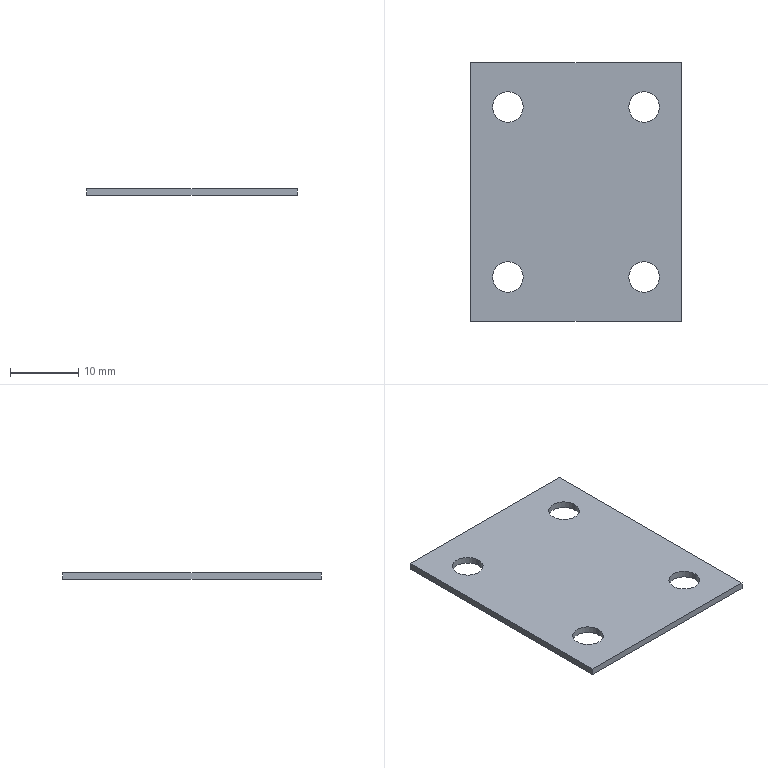Part | SolidWorks | features Extrusion 1 | 1 solid | 14 faces | box 31 x 38 x 1 mm | volume 1114 mm3 | cylinder 8 | plane 6 | commonest cylinder face diameters 4.5 x8
STEP:
#1=CARTESIAN_POINT('',(-12.25,-12.5,1.));
#2=VERTEX_POINT('',#1);
#3=CARTESIAN_POINT('',(-7.75,-12.5,1.));
#4=VERTEX_POINT('',#3);
#5=CARTESIAN_POINT('',(-10.,-12.5,1.));
#6=DIRECTION('',(0.,0.,1.));
#7=DIRECTION('',(1.,0.,0.));
#8=AXIS2_PLACEMENT_3D('',#5,#6,#7);
#9=CIRCLE('',#8,2.25);
#10=EDGE_CURVE('',#2,#4,#9,.T.);
#11=ORIENTED_EDGE('',*,*,#10,.T.);
#12=CARTESIAN_POINT('',(-7.75,-12.5,0.));
#13=VERTEX_POINT('',#12);
#14=CARTESIAN_POINT('',(-7.75,-12.5,1.));
#15=DIRECTION('',(0.,0.,-1.));
#16=VECTOR('',#15,1000.);
#17=LINE('',#14,#16);
#18=EDGE_CURVE('',#4,#13,#17,.T.);
#19=ORIENTED_EDGE('',*,*,#18,.T.);
#20=CARTESIAN_POINT('',(-12.25,-12.5,0.));
#21=VERTEX_POINT('',#20);
#22=CARTESIAN_POINT('',(-10.,-12.5,0.));
#23=DIRECTION('',(0.,0.,1.));
#24=DIRECTION('',(1.,0.,0.));
#25=AXIS2_PLACEMENT_3D('',#22,#23,#24);
#26=CIRCLE('',#25,2.25);
#27=EDGE_CURVE('',#21,#13,#26,.T.);
#28=ORIENTED_EDGE('',*,*,#27,.F.);
#29=CARTESIAN_POINT('',(-12.25,-12.5,1.));
#30=DIRECTION('',(0.,0.,-1.));
#31=VECTOR('',#30,1000.);
#32=LINE('',#29,#31);
#33=EDGE_CURVE('',#2,#21,#32,.T.);
#34=ORIENTED_EDGE('',*,*,#33,.F.);
#35=EDGE_LOOP('',(#11,#19,#28,#34));
#36=FACE_OUTER_BOUND('',#35,.T.);
#37=CARTESIAN_POINT('',(-10.,-12.5,1.));
#38=DIRECTION('',(0.,0.,-1.));
#39=DIRECTION('',(-1.,0.,0.));
#40=AXIS2_PLACEMENT_3D('',#37,#38,#39);
#41=CYLINDRICAL_SURFACE('',#40,2.25);
#42=ADVANCED_FACE('',(#36),#41,.F.);
#43=CARTESIAN_POINT('',(7.75,-12.5,1.));
#44=VERTEX_POINT('',#43);
#45=CARTESIAN_POINT('',(12.25,-12.5,1.));
#46=VERTEX_POINT('',#45);
#47=CARTESIAN_POINT('',(10.,-12.5,1.));
#48=DIRECTION('',(0.,0.,1.));
#49=DIRECTION('',(1.,0.,0.));
#50=AXIS2_PLACEMENT_3D('',#47,#48,#49);
#51=CIRCLE('',#50,2.25);
#52=EDGE_CURVE('',#44,#46,#51,.T.);
#53=ORIENTED_EDGE('',*,*,#52,.T.);
#54=CARTESIAN_POINT('',(12.25,-12.5,0.));
#55=VERTEX_POINT('',#54);
#56=CARTESIAN_POINT('',(12.25,-12.5,1.));
#57=DIRECTION('',(0.,0.,-1.));
#58=VECTOR('',#57,1000.);
#59=LINE('',#56,#58);
#60=EDGE_CURVE('',#46,#55,#59,.T.);
#61=ORIENTED_EDGE('',*,*,#60,.T.);
#62=CARTESIAN_POINT('',(7.75,-12.5,0.));
#63=VERTEX_POINT('',#62);
#64=CARTESIAN_POINT('',(10.,-12.5,0.));
#65=DIRECTION('',(0.,0.,1.));
#66=DIRECTION('',(1.,0.,0.));
#67=AXIS2_PLACEMENT_3D('',#64,#65,#66);
#68=CIRCLE('',#67,2.25);
#69=EDGE_CURVE('',#63,#55,#68,.T.);
#70=ORIENTED_EDGE('',*,*,#69,.F.);
#71=CARTESIAN_POINT('',(7.75,-12.5,1.));
#72=DIRECTION('',(0.,0.,-1.));
#73=VECTOR('',#72,1000.);
#74=LINE('',#71,#73);
#75=EDGE_CURVE('',#44,#63,#74,.T.);
#76=ORIENTED_EDGE('',*,*,#75,.F.);
#77=EDGE_LOOP('',(#53,#61,#70,#76));
#78=FACE_OUTER_BOUND('',#77,.T.);
#79=CARTESIAN_POINT('',(10.,-12.5,1.));
#80=DIRECTION('',(0.,0.,-1.));
#81=DIRECTION('',(-1.,0.,0.));
#82=AXIS2_PLACEMENT_3D('',#79,#80,#81);
#83=CYLINDRICAL_SURFACE('',#82,2.25);
#84=ADVANCED_FACE('',(#78),#83,.F.);
#85=CARTESIAN_POINT('',(7.75,12.5,1.));
#86=VERTEX_POINT('',#85);
#87=CARTESIAN_POINT('',(12.25,12.5,1.));
#88=VERTEX_POINT('',#87);
#89=CARTESIAN_POINT('',(10.,12.5,1.));
#90=DIRECTION('',(0.,0.,1.));
#91=DIRECTION('',(1.,0.,0.));
#92=AXIS2_PLACEMENT_3D('',#89,#90,#91);
#93=CIRCLE('',#92,2.25);
#94=EDGE_CURVE('',#86,#88,#93,.T.);
#95=ORIENTED_EDGE('',*,*,#94,.T.);
#96=CARTESIAN_POINT('',(12.25,12.5,0.));
#97=VERTEX_POINT('',#96);
#98=CARTESIAN_POINT('',(12.25,12.5,1.));
#99=DIRECTION('',(0.,0.,-1.));
#100=VECTOR('',#99,1000.);
#101=LINE('',#98,#100);
#102=EDGE_CURVE('',#88,#97,#101,.T.);
#103=ORIENTED_EDGE('',*,*,#102,.T.);
#104=CARTESIAN_POINT('',(7.75,12.5,0.));
#105=VERTEX_POINT('',#104);
#106=CARTESIAN_POINT('',(10.,12.5,0.));
#107=DIRECTION('',(0.,0.,1.));
#108=DIRECTION('',(1.,0.,0.));
#109=AXIS2_PLACEMENT_3D('',#106,#107,#108);
#110=CIRCLE('',#109,2.25);
#111=EDGE_CURVE('',#105,#97,#110,.T.);
#112=ORIENTED_EDGE('',*,*,#111,.F.);
#113=CARTESIAN_POINT('',(7.75,12.5,1.));
#114=DIRECTION('',(0.,0.,-1.));
#115=VECTOR('',#114,1000.);
#116=LINE('',#113,#115);
#117=EDGE_CURVE('',#86,#105,#116,.T.);
#118=ORIENTED_EDGE('',*,*,#117,.F.);
#119=EDGE_LOOP('',(#95,#103,#112,#118));
#120=FACE_OUTER_BOUND('',#119,.T.);
#121=CARTESIAN_POINT('',(10.,12.5,1.));
#122=DIRECTION('',(0.,0.,-1.));
#123=DIRECTION('',(-1.,0.,0.));
#124=AXIS2_PLACEMENT_3D('',#121,#122,#123);
#125=CYLINDRICAL_SURFACE('',#124,2.25);
#126=ADVANCED_FACE('',(#120),#125,.F.);
#127=CARTESIAN_POINT('',(-12.25,12.5,1.));
#128=VERTEX_POINT('',#127);
#129=CARTESIAN_POINT('',(-7.75,12.5,1.));
#130=VERTEX_POINT('',#129);
#131=CARTESIAN_POINT('',(-10.,12.5,1.));
#132=DIRECTION('',(0.,0.,1.));
#133=DIRECTION('',(1.,0.,0.));
#134=AXIS2_PLACEMENT_3D('',#131,#132,#133);
#135=CIRCLE('',#134,2.25);
#136=EDGE_CURVE('',#128,#130,#135,.T.);
#137=ORIENTED_EDGE('',*,*,#136,.T.);
#138=CARTESIAN_POINT('',(-7.75,12.5,0.));
#139=VERTEX_POINT('',#138);
#140=CARTESIAN_POINT('',(-7.75,12.5,1.));
#141=DIRECTION('',(0.,0.,-1.));
#142=VECTOR('',#141,1000.);
#143=LINE('',#140,#142);
#144=EDGE_CURVE('',#130,#139,#143,.T.);
#145=ORIENTED_EDGE('',*,*,#144,.T.);
#146=CARTESIAN_POINT('',(-12.25,12.5,0.));
#147=VERTEX_POINT('',#146);
#148=CARTESIAN_POINT('',(-10.,12.5,0.));
#149=DIRECTION('',(0.,0.,1.));
#150=DIRECTION('',(1.,0.,0.));
#151=AXIS2_PLACEMENT_3D('',#148,#149,#150);
#152=CIRCLE('',#151,2.25);
#153=EDGE_CURVE('',#147,#139,#152,.T.);
#154=ORIENTED_EDGE('',*,*,#153,.F.);
#155=CARTESIAN_POINT('',(-12.25,12.5,1.));
#156=DIRECTION('',(0.,0.,-1.));
#157=VECTOR('',#156,1000.);
#158=LINE('',#155,#157);
#159=EDGE_CURVE('',#128,#147,#158,.T.);
#160=ORIENTED_EDGE('',*,*,#159,.F.);
#161=EDGE_LOOP('',(#137,#145,#154,#160));
#162=FACE_OUTER_BOUND('',#161,.T.);
#163=CARTESIAN_POINT('',(-10.,12.5,1.));
#164=DIRECTION('',(0.,0.,-1.));
#165=DIRECTION('',(-1.,0.,0.));
#166=AXIS2_PLACEMENT_3D('',#163,#164,#165);
#167=CYLINDRICAL_SURFACE('',#166,2.25);
#168=ADVANCED_FACE('',(#162),#167,.F.);
#169=ORIENTED_EDGE('',*,*,#52,.F.);
#170=CARTESIAN_POINT('',(10.,-12.5,1.));
#171=DIRECTION('',(0.,0.,1.));
#172=DIRECTION('',(1.,0.,0.));
#173=AXIS2_PLACEMENT_3D('',#170,#171,#172);
#174=CIRCLE('',#173,2.25);
#175=EDGE_CURVE('',#46,#44,#174,.T.);
#176=ORIENTED_EDGE('',*,*,#175,.F.);
#177=EDGE_LOOP('',(#169,#176));
#178=FACE_BOUND('',#177,.T.);
#179=ORIENTED_EDGE('',*,*,#136,.F.);
#180=CARTESIAN_POINT('',(-10.,12.5,1.));
#181=DIRECTION('',(0.,0.,1.));
#182=DIRECTION('',(1.,0.,0.));
#183=AXIS2_PLACEMENT_3D('',#180,#181,#182);
#184=CIRCLE('',#183,2.25);
#185=EDGE_CURVE('',#130,#128,#184,.T.);
#186=ORIENTED_EDGE('',*,*,#185,.F.);
#187=EDGE_LOOP('',(#179,#186));
#188=FACE_BOUND('',#187,.T.);
#189=CARTESIAN_POINT('',(-15.5,19.,1.));
#190=VERTEX_POINT('',#189);
#191=CARTESIAN_POINT('',(-15.5,-19.,1.));
#192=VERTEX_POINT('',#191);
#193=CARTESIAN_POINT('',(-15.5,-19.,1.));
#194=DIRECTION('',(0.,-1.,0.));
#195=VECTOR('',#194,1000.);
#196=LINE('',#193,#195);
#197=EDGE_CURVE('',#190,#192,#196,.T.);
#198=ORIENTED_EDGE('',*,*,#197,.T.);
#199=CARTESIAN_POINT('',(15.5,-19.,1.));
#200=VERTEX_POINT('',#199);
#201=CARTESIAN_POINT('',(15.5,-19.,1.));
#202=DIRECTION('',(1.,0.,0.));
#203=VECTOR('',#202,1000.);
#204=LINE('',#201,#203);
#205=EDGE_CURVE('',#192,#200,#204,.T.);
#206=ORIENTED_EDGE('',*,*,#205,.T.);
#207=CARTESIAN_POINT('',(15.5,19.,1.));
#208=VERTEX_POINT('',#207);
#209=CARTESIAN_POINT('',(15.5,-19.,1.));
#210=DIRECTION('',(0.,1.,0.));
#211=VECTOR('',#210,1000.);
#212=LINE('',#209,#211);
#213=EDGE_CURVE('',#200,#208,#212,.T.);
#214=ORIENTED_EDGE('',*,*,#213,.T.);
#215=CARTESIAN_POINT('',(15.5,19.,1.));
#216=DIRECTION('',(-1.,0.,0.));
#217=VECTOR('',#216,1000.);
#218=LINE('',#215,#217);
#219=EDGE_CURVE('',#208,#190,#218,.T.);
#220=ORIENTED_EDGE('',*,*,#219,.T.);
#221=EDGE_LOOP('',(#198,#206,#214,#220));
#222=FACE_OUTER_BOUND('',#221,.T.);
#223=ORIENTED_EDGE('',*,*,#94,.F.);
#224=CARTESIAN_POINT('',(10.,12.5,1.));
#225=DIRECTION('',(0.,0.,1.));
#226=DIRECTION('',(1.,0.,0.));
#227=AXIS2_PLACEMENT_3D('',#224,#225,#226);
#228=CIRCLE('',#227,2.25);
#229=EDGE_CURVE('',#88,#86,#228,.T.);
#230=ORIENTED_EDGE('',*,*,#229,.F.);
#231=EDGE_LOOP('',(#223,#230));
#232=FACE_BOUND('',#231,.T.);
#233=ORIENTED_EDGE('',*,*,#10,.F.);
#234=CARTESIAN_POINT('',(-10.,-12.5,1.));
#235=DIRECTION('',(0.,0.,1.));
#236=DIRECTION('',(1.,0.,0.));
#237=AXIS2_PLACEMENT_3D('',#234,#235,#236);
#238=CIRCLE('',#237,2.25);
#239=EDGE_CURVE('',#4,#2,#238,.T.);
#240=ORIENTED_EDGE('',*,*,#239,.F.);
#241=EDGE_LOOP('',(#233,#240));
#242=FACE_BOUND('',#241,.T.);
#243=CARTESIAN_POINT('',(0.,0.,1.));
#244=DIRECTION('',(0.,0.,1.));
#245=DIRECTION('',(1.,0.,0.));
#246=AXIS2_PLACEMENT_3D('',#243,#244,#245);
#247=PLANE('',#246);
#248=ADVANCED_FACE('',(#178,#188,#222,#232,#242),#247,.T.);
#249=CARTESIAN_POINT('',(-15.5,19.,0.));
#250=VERTEX_POINT('',#249);
#251=CARTESIAN_POINT('',(-15.5,-19.,0.));
#252=VERTEX_POINT('',#251);
#253=CARTESIAN_POINT('',(-15.5,-19.,0.));
#254=DIRECTION('',(0.,-1.,0.));
#255=VECTOR('',#254,1000.);
#256=LINE('',#253,#255);
#257=EDGE_CURVE('',#250,#252,#256,.T.);
#258=ORIENTED_EDGE('',*,*,#257,.F.);
#259=CARTESIAN_POINT('',(15.5,19.,0.));
#260=VERTEX_POINT('',#259);
#261=CARTESIAN_POINT('',(15.5,19.,0.));
#262=DIRECTION('',(-1.,0.,0.));
#263=VECTOR('',#262,1000.);
#264=LINE('',#261,#263);
#265=EDGE_CURVE('',#260,#250,#264,.T.);
#266=ORIENTED_EDGE('',*,*,#265,.F.);
#267=CARTESIAN_POINT('',(15.5,-19.,0.));
#268=VERTEX_POINT('',#267);
#269=CARTESIAN_POINT('',(15.5,-19.,0.));
#270=DIRECTION('',(0.,1.,0.));
#271=VECTOR('',#270,1000.);
#272=LINE('',#269,#271);
#273=EDGE_CURVE('',#268,#260,#272,.T.);
#274=ORIENTED_EDGE('',*,*,#273,.F.);
#275=CARTESIAN_POINT('',(15.5,-19.,0.));
#276=DIRECTION('',(1.,0.,0.));
#277=VECTOR('',#276,1000.);
#278=LINE('',#275,#277);
#279=EDGE_CURVE('',#252,#268,#278,.T.);
#280=ORIENTED_EDGE('',*,*,#279,.F.);
#281=EDGE_LOOP('',(#258,#266,#274,#280));
#282=FACE_OUTER_BOUND('',#281,.T.);
#283=ORIENTED_EDGE('',*,*,#153,.T.);
#284=CARTESIAN_POINT('',(-10.,12.5,0.));
#285=DIRECTION('',(0.,0.,1.));
#286=DIRECTION('',(1.,0.,0.));
#287=AXIS2_PLACEMENT_3D('',#284,#285,#286);
#288=CIRCLE('',#287,2.25);
#289=EDGE_CURVE('',#139,#147,#288,.T.);
#290=ORIENTED_EDGE('',*,*,#289,.T.);
#291=EDGE_LOOP('',(#283,#290));
#292=FACE_BOUND('',#291,.T.);
#293=ORIENTED_EDGE('',*,*,#111,.T.);
#294=CARTESIAN_POINT('',(10.,12.5,0.));
#295=DIRECTION('',(0.,0.,1.));
#296=DIRECTION('',(1.,0.,0.));
#297=AXIS2_PLACEMENT_3D('',#294,#295,#296);
#298=CIRCLE('',#297,2.25);
#299=EDGE_CURVE('',#97,#105,#298,.T.);
#300=ORIENTED_EDGE('',*,*,#299,.T.);
#301=EDGE_LOOP('',(#293,#300));
#302=FACE_BOUND('',#301,.T.);
#303=ORIENTED_EDGE('',*,*,#69,.T.);
#304=CARTESIAN_POINT('',(10.,-12.5,0.));
#305=DIRECTION('',(0.,0.,1.));
#306=DIRECTION('',(1.,0.,0.));
#307=AXIS2_PLACEMENT_3D('',#304,#305,#306);
#308=CIRCLE('',#307,2.25);
#309=EDGE_CURVE('',#55,#63,#308,.T.);
#310=ORIENTED_EDGE('',*,*,#309,.T.);
#311=EDGE_LOOP('',(#303,#310));
#312=FACE_BOUND('',#311,.T.);
#313=ORIENTED_EDGE('',*,*,#27,.T.);
#314=CARTESIAN_POINT('',(-10.,-12.5,0.));
#315=DIRECTION('',(0.,0.,1.));
#316=DIRECTION('',(1.,0.,0.));
#317=AXIS2_PLACEMENT_3D('',#314,#315,#316);
#318=CIRCLE('',#317,2.25);
#319=EDGE_CURVE('',#13,#21,#318,.T.);
#320=ORIENTED_EDGE('',*,*,#319,.T.);
#321=EDGE_LOOP('',(#313,#320));
#322=FACE_BOUND('',#321,.T.);
#323=CARTESIAN_POINT('',(0.,0.,0.));
#324=DIRECTION('',(0.,0.,1.));
#325=DIRECTION('',(1.,0.,0.));
#326=AXIS2_PLACEMENT_3D('',#323,#324,#325);
#327=PLANE('',#326);
#328=ADVANCED_FACE('',(#282,#292,#302,#312,#322),#327,.F.);
#329=ORIENTED_EDGE('',*,*,#257,.T.);
#330=CARTESIAN_POINT('',(-15.5,-19.,1.));
#331=DIRECTION('',(0.,0.,-1.));
#332=VECTOR('',#331,1000.);
#333=LINE('',#330,#332);
#334=EDGE_CURVE('',#192,#252,#333,.T.);
#335=ORIENTED_EDGE('',*,*,#334,.F.);
#336=ORIENTED_EDGE('',*,*,#197,.F.);
#337=CARTESIAN_POINT('',(-15.5,19.,1.));
#338=DIRECTION('',(0.,0.,-1.));
#339=VECTOR('',#338,1000.);
#340=LINE('',#337,#339);
#341=EDGE_CURVE('',#190,#250,#340,.T.);
#342=ORIENTED_EDGE('',*,*,#341,.T.);
#343=EDGE_LOOP('',(#329,#335,#336,#342));
#344=FACE_OUTER_BOUND('',#343,.T.);
#345=CARTESIAN_POINT('',(-15.5,-19.,1.));
#346=DIRECTION('',(1.,0.,0.));
#347=DIRECTION('',(0.,1.,0.));
#348=AXIS2_PLACEMENT_3D('',#345,#346,#347);
#349=PLANE('',#348);
#350=ADVANCED_FACE('',(#344),#349,.F.);
#351=ORIENTED_EDGE('',*,*,#279,.T.);
#352=CARTESIAN_POINT('',(15.5,-19.,1.));
#353=DIRECTION('',(0.,0.,-1.));
#354=VECTOR('',#353,1000.);
#355=LINE('',#352,#354);
#356=EDGE_CURVE('',#200,#268,#355,.T.);
#357=ORIENTED_EDGE('',*,*,#356,.F.);
#358=ORIENTED_EDGE('',*,*,#205,.F.);
#359=ORIENTED_EDGE('',*,*,#334,.T.);
#360=EDGE_LOOP('',(#351,#357,#358,#359));
#361=FACE_OUTER_BOUND('',#360,.T.);
#362=CARTESIAN_POINT('',(15.5,-19.,1.));
#363=DIRECTION('',(0.,1.,0.));
#364=DIRECTION('',(0.,0.,1.));
#365=AXIS2_PLACEMENT_3D('',#362,#363,#364);
#366=PLANE('',#365);
#367=ADVANCED_FACE('',(#361),#366,.F.);
#368=ORIENTED_EDGE('',*,*,#273,.T.);
#369=CARTESIAN_POINT('',(15.5,19.,1.));
#370=DIRECTION('',(0.,0.,-1.));
#371=VECTOR('',#370,1000.);
#372=LINE('',#369,#371);
#373=EDGE_CURVE('',#208,#260,#372,.T.);
#374=ORIENTED_EDGE('',*,*,#373,.F.);
#375=ORIENTED_EDGE('',*,*,#213,.F.);
#376=ORIENTED_EDGE('',*,*,#356,.T.);
#377=EDGE_LOOP('',(#368,#374,#375,#376));
#378=FACE_OUTER_BOUND('',#377,.T.);
#379=CARTESIAN_POINT('',(15.5,-19.,1.));
#380=DIRECTION('',(-1.,0.,0.));
#381=DIRECTION('',(0.,0.,1.));
#382=AXIS2_PLACEMENT_3D('',#379,#380,#381);
#383=PLANE('',#382);
#384=ADVANCED_FACE('',(#378),#383,.F.);
#385=ORIENTED_EDGE('',*,*,#265,.T.);
#386=ORIENTED_EDGE('',*,*,#341,.F.);
#387=ORIENTED_EDGE('',*,*,#219,.F.);
#388=ORIENTED_EDGE('',*,*,#373,.T.);
#389=EDGE_LOOP('',(#385,#386,#387,#388));
#390=FACE_OUTER_BOUND('',#389,.T.);
#391=CARTESIAN_POINT('',(15.5,19.,1.));
#392=DIRECTION('',(0.,-1.,0.));
#393=DIRECTION('',(1.,0.,0.));
#394=AXIS2_PLACEMENT_3D('',#391,#392,#393);
#395=PLANE('',#394);
#396=ADVANCED_FACE('',(#390),#395,.F.);
#397=ORIENTED_EDGE('',*,*,#144,.F.);
#398=ORIENTED_EDGE('',*,*,#185,.T.);
#399=ORIENTED_EDGE('',*,*,#159,.T.);
#400=ORIENTED_EDGE('',*,*,#289,.F.);
#401=EDGE_LOOP('',(#397,#398,#399,#400));
#402=FACE_OUTER_BOUND('',#401,.T.);
#403=CARTESIAN_POINT('',(-10.,12.5,1.));
#404=DIRECTION('',(0.,0.,-1.));
#405=DIRECTION('',(-1.,0.,0.));
#406=AXIS2_PLACEMENT_3D('',#403,#404,#405);
#407=CYLINDRICAL_SURFACE('',#406,2.25);
#408=ADVANCED_FACE('',(#402),#407,.F.);
#409=ORIENTED_EDGE('',*,*,#102,.F.);
#410=ORIENTED_EDGE('',*,*,#229,.T.);
#411=ORIENTED_EDGE('',*,*,#117,.T.);
#412=ORIENTED_EDGE('',*,*,#299,.F.);
#413=EDGE_LOOP('',(#409,#410,#411,#412));
#414=FACE_OUTER_BOUND('',#413,.T.);
#415=CARTESIAN_POINT('',(10.,12.5,1.));
#416=DIRECTION('',(0.,0.,-1.));
#417=DIRECTION('',(-1.,0.,0.));
#418=AXIS2_PLACEMENT_3D('',#415,#416,#417);
#419=CYLINDRICAL_SURFACE('',#418,2.25);
#420=ADVANCED_FACE('',(#414),#419,.F.);
#421=ORIENTED_EDGE('',*,*,#60,.F.);
#422=ORIENTED_EDGE('',*,*,#175,.T.);
#423=ORIENTED_EDGE('',*,*,#75,.T.);
#424=ORIENTED_EDGE('',*,*,#309,.F.);
#425=EDGE_LOOP('',(#421,#422,#423,#424));
#426=FACE_OUTER_BOUND('',#425,.T.);
#427=CARTESIAN_POINT('',(10.,-12.5,1.));
#428=DIRECTION('',(0.,0.,-1.));
#429=DIRECTION('',(-1.,0.,0.));
#430=AXIS2_PLACEMENT_3D('',#427,#428,#429);
#431=CYLINDRICAL_SURFACE('',#430,2.25);
#432=ADVANCED_FACE('',(#426),#431,.F.);
#433=ORIENTED_EDGE('',*,*,#18,.F.);
#434=ORIENTED_EDGE('',*,*,#239,.T.);
#435=ORIENTED_EDGE('',*,*,#33,.T.);
#436=ORIENTED_EDGE('',*,*,#319,.F.);
#437=EDGE_LOOP('',(#433,#434,#435,#436));
#438=FACE_OUTER_BOUND('',#437,.T.);
#439=CARTESIAN_POINT('',(-10.,-12.5,1.));
#440=DIRECTION('',(0.,0.,-1.));
#441=DIRECTION('',(-1.,0.,0.));
#442=AXIS2_PLACEMENT_3D('',#439,#440,#441);
#443=CYLINDRICAL_SURFACE('',#442,2.25);
#444=ADVANCED_FACE('',(#438),#443,.F.);
#445=CLOSED_SHELL('',(#42,#84,#126,#168,#248,#328,#350,#367,#384,#396,#408,#420,#432,#444));
#446=MANIFOLD_SOLID_BREP('',#445);
#447=CARTESIAN_POINT('',(0.,0.,0.));
#448=DIRECTION('',(0.,0.,1.));
#449=DIRECTION('',(1.,0.,0.));
#450=AXIS2_PLACEMENT_3D('',#447,#448,#449);
#451=(LENGTH_UNIT()NAMED_UNIT(*)SI_UNIT(.MILLI.,.METRE.));
#452=UNCERTAINTY_MEASURE_WITH_UNIT(LENGTH_MEASURE(0.00001),#451,'','');
#453=(NAMED_UNIT(*)PLANE_ANGLE_UNIT()SI_UNIT($,.RADIAN.));
#454=(NAMED_UNIT(*)SI_UNIT($,.STERADIAN.)SOLID_ANGLE_UNIT());
#455=(GEOMETRIC_REPRESENTATION_CONTEXT(3)GLOBAL_UNCERTAINTY_ASSIGNED_CONTEXT((#452))GLOBAL_UNIT_ASSIGNED_CONTEXT((#451,#453,#454))REPRESENTATION_CONTEXT('',''));
#456=ADVANCED_BREP_SHAPE_REPRESENTATION('',(#446,#450),#455);